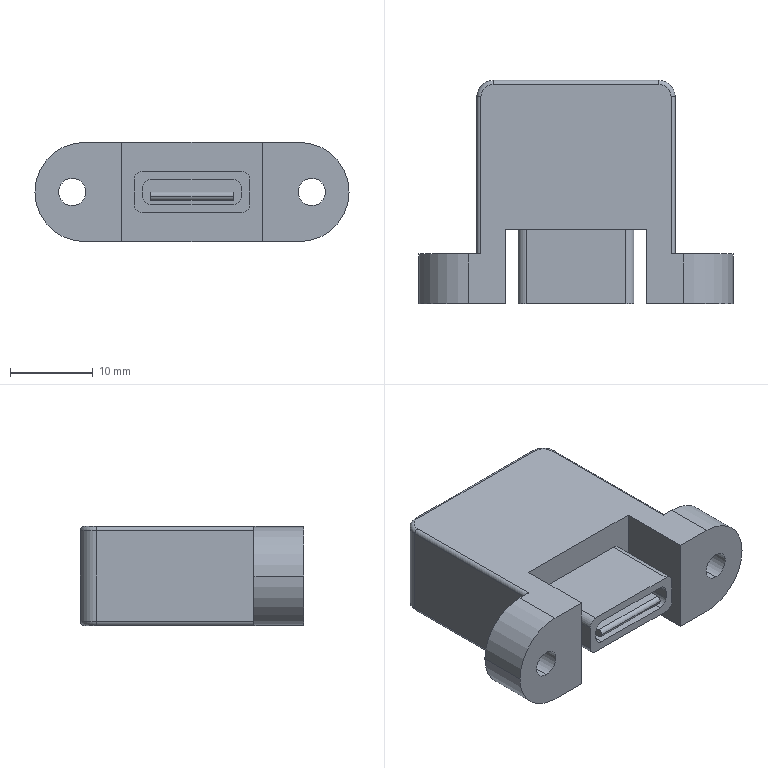Part | STEP file | USB interface | 1 solid | 56 faces | box 38 x 27 x 12 mm | volume 7027 mm3 | cylinder 26 | plane 26 | torus 4 | commonest cylinder face diameters 1 x8 2 x8 3.3 x4 12 x4 4 x2